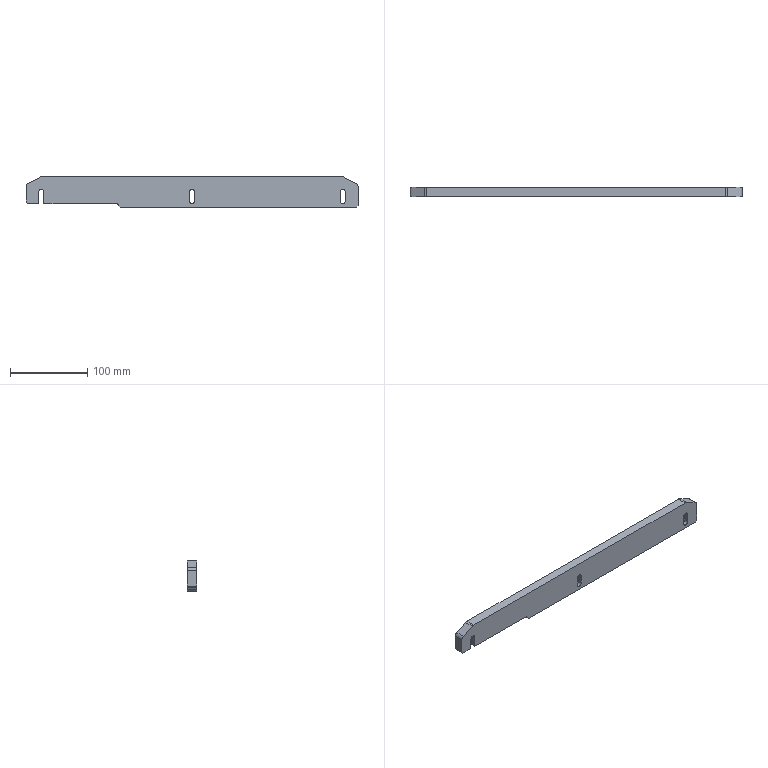CAM job | NX | 3+2 milling | part box 430.5 x 12 x 40 mm | stock box 435.5 x 15 x 45 mm
Tools:
number,name,description,diameter,corner_radius,flute_length,length,flutes
4,D4,平底铣刀-粗,4.0,0.0,25.0,75.0,2
6,D6,平底铣刀-粗,6.0,0.0,25.0,75.0,2
9,D10,平底铣刀-粗,10.0,0.0,35.0,75.0,2
11,D4-J,平底铣刀-精,4.0,0.0,50.0,75.0,2
7,D6-J,平底铣刀-精,6.0,0.0,25.0,75.0,2
1,D80R0.8飞刀,圆鼻刀-粗,80.0,0.8,50.0,75.0,2
1,D80R0.8飞刀-J,圆鼻刀-精,80.0,0.8,50.0,75.0,2
2,D6倒角刀,倒角刀,6.0,0.0,3.0,25.0,2
Operations:
program,operation,operation_type,tool,method,geometry_group,spindle_rpm,surface_speed,feed_per_tooth,feed_cut,feed_plunge,cut_length_mm,path_length_mm,cut_time_min,machine_time_min
B,底壁铣飞面一刀开粗_COPY,VolumeBased25DMillingOperation,D80R0.8飞刀,分层开粗-切深K-步距G,W-B,2800.0,703.696,0.5357,3000.0,100.0,3232.396,6189.11,1.077,1.373
B,底壁铣飞面一刀精光_COPY,VolumeBased25DMillingOperation,D80R0.8飞刀-J,侧刃精光-切深K-步距G,W-B,4000.0,1005.28,0.125,1000.0,100.0,538.537,634.537,0.5385,0.5481
B,C0.3平面去毛刺6X45L__COPY,SurfaceContour,D6倒角刀,爬面_倒角-切深0-步距G,W-B,8000.0,150.796,0.0938,1500.0,90.0,1048.665,1405.508,0.6995,0.7352
A,顶面,FaceMilling,D80R0.8飞刀,侧刃精光-切深K-步距G,W-A,4000.0,1005.31,0.125,1000.0,100.0,524.5,560.5,0.5245,0.5281
A,外形粗_2,VolumeBased25DMillingOperation,D10,METHOD,W-A,8000.0,251.327,0.3125,5000.0,80.0,16179.621,16230.421,3.236,3.241
A,盲腰槽粗,VolumeBased25DMillingOperation,D6,METHOD,W-A,6000.0,113.097,0.1667,2000.0,100.0,2035.196,2321.047,1.018,1.046
A,底壁铣分层开粗-中_COPY,VolumeBased25DMillingOperation,D6,分层开粗-切深K-步距G,W-A,8000.0,150.792,0.1875,3000.0,100.0,738.357,825.645,0.2461,0.2548
A,通腰槽粗_1,VolumeBased25DMillingOperation,D4,METHOD,W-A,6000.0,75.398,0.1,1200.0,100.0,1580.037,1890.288,1.317,1.348
A,腰槽精_3,VolumeBased25DMillingOperation,D4-J,METHOD,W-A,6000.0,113.0,0.0417,500.0,100.0,137.586,472.137,0.2752,0.3086
A,外形侧面,ZLevelMilling,D6-J,METHOD,W-A,9000.0,84.823,0.1389,2500.0,80.0,1017.133,1175.823,0.4072,0.423
A,腰槽精,VolumeBased25DMillingOperation,D6-J,METHOD,W-A,6000.0,113.0,0.0667,600.0,100.0,167.745,485.597,0.2796,0.3114
A,底侧精_3,VolumeBased25DMillingOperation,D6-J,METHOD,W-A,6000.0,113.0,0.2083,1200.0,100.0,47.596,100.196,0.0397,0.0449
A,仅选体,SurfaceContour,D6倒角刀,METHOD,W-A,8000.0,150.796,0.1875,3000.0,100.0,1092.201,1423.403,0.3641,0.3972
A,外形半精_2,VolumeBased25DMillingOperation,D6-J,METHOD,W-A,8000.0,251.327,0.0625,1000.0,100.0,977.148,1040.748,0.9771,0.9835